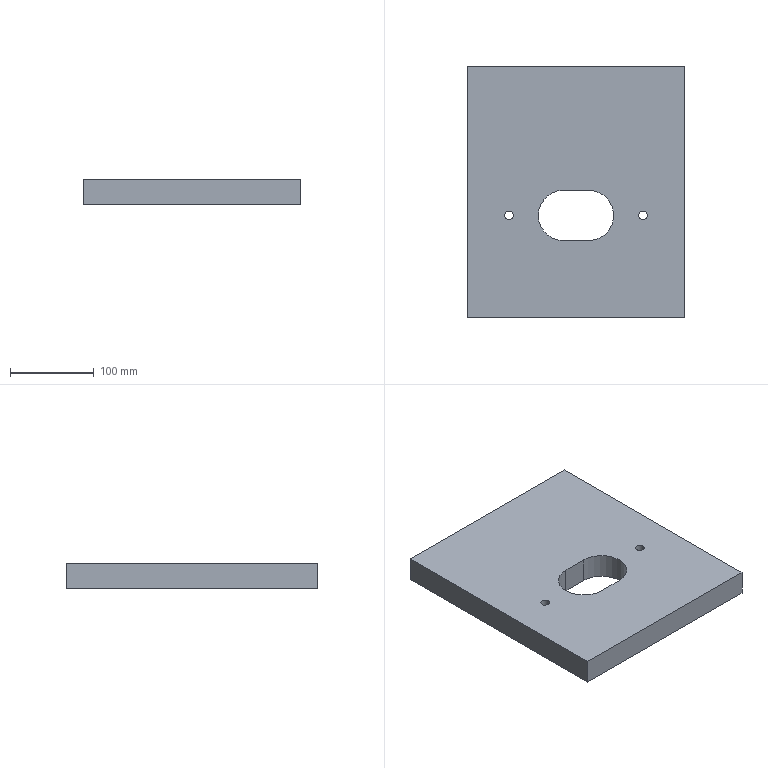Part | SolidWorks | features 3DProfileFeature 1, Extrusion 1, HoleWzd 1 | 1 solid | 15 faces | box 260 x 300 x 30 mm | volume 2196274 mm3 | plane 8 | cylinder 7 | commonest cylinder face diameters 10.2 x4 60 x3
STEP:
#1=CARTESIAN_POINT('',(44.9,122.,0.));
#2=VERTEX_POINT('',#1);
#3=CARTESIAN_POINT('',(55.1,122.,0.));
#4=VERTEX_POINT('',#3);
#5=CARTESIAN_POINT('',(50.,122.,0.));
#6=DIRECTION('',(0.,0.,1.));
#7=DIRECTION('',(1.,0.,0.));
#8=AXIS2_PLACEMENT_3D('',#5,#6,#7);
#9=CIRCLE('',#8,5.1);
#10=EDGE_CURVE('',#2,#4,#9,.T.);
#11=ORIENTED_EDGE('',*,*,#10,.F.);
#12=CARTESIAN_POINT('',(44.9,122.,30.));
#13=VERTEX_POINT('',#12);
#14=CARTESIAN_POINT('',(44.9,122.,30.));
#15=DIRECTION('',(0.,0.,1.));
#16=VECTOR('',#15,1000.);
#17=LINE('',#14,#16);
#18=EDGE_CURVE('',#2,#13,#17,.T.);
#19=ORIENTED_EDGE('',*,*,#18,.T.);
#20=CARTESIAN_POINT('',(55.1,122.,30.));
#21=VERTEX_POINT('',#20);
#22=CARTESIAN_POINT('',(50.,122.,30.));
#23=DIRECTION('',(0.,0.,1.));
#24=DIRECTION('',(1.,0.,0.));
#25=AXIS2_PLACEMENT_3D('',#22,#23,#24);
#26=CIRCLE('',#25,5.1);
#27=EDGE_CURVE('',#13,#21,#26,.T.);
#28=ORIENTED_EDGE('',*,*,#27,.T.);
#29=CARTESIAN_POINT('',(55.1,122.,30.));
#30=DIRECTION('',(0.,0.,1.));
#31=VECTOR('',#30,1000.);
#32=LINE('',#29,#31);
#33=EDGE_CURVE('',#4,#21,#32,.T.);
#34=ORIENTED_EDGE('',*,*,#33,.F.);
#35=EDGE_LOOP('',(#11,#19,#28,#34));
#36=FACE_OUTER_BOUND('',#35,.T.);
#37=CARTESIAN_POINT('',(50.,122.,30.));
#38=DIRECTION('',(0.,0.,1.));
#39=DIRECTION('',(1.,0.,0.));
#40=AXIS2_PLACEMENT_3D('',#37,#38,#39);
#41=CYLINDRICAL_SURFACE('',#40,5.1);
#42=ADVANCED_FACE('',(#36),#41,.F.);
#43=CARTESIAN_POINT('',(204.9,122.,0.));
#44=VERTEX_POINT('',#43);
#45=CARTESIAN_POINT('',(215.1,122.,0.));
#46=VERTEX_POINT('',#45);
#47=CARTESIAN_POINT('',(210.,122.,0.));
#48=DIRECTION('',(0.,0.,1.));
#49=DIRECTION('',(1.,0.,0.));
#50=AXIS2_PLACEMENT_3D('',#47,#48,#49);
#51=CIRCLE('',#50,5.1);
#52=EDGE_CURVE('',#44,#46,#51,.T.);
#53=ORIENTED_EDGE('',*,*,#52,.F.);
#54=CARTESIAN_POINT('',(204.9,122.,30.));
#55=VERTEX_POINT('',#54);
#56=CARTESIAN_POINT('',(204.9,122.,30.));
#57=DIRECTION('',(0.,0.,1.));
#58=VECTOR('',#57,1000.);
#59=LINE('',#56,#58);
#60=EDGE_CURVE('',#44,#55,#59,.T.);
#61=ORIENTED_EDGE('',*,*,#60,.T.);
#62=CARTESIAN_POINT('',(215.1,122.,30.));
#63=VERTEX_POINT('',#62);
#64=CARTESIAN_POINT('',(210.,122.,30.));
#65=DIRECTION('',(0.,0.,1.));
#66=DIRECTION('',(1.,0.,0.));
#67=AXIS2_PLACEMENT_3D('',#64,#65,#66);
#68=CIRCLE('',#67,5.1);
#69=EDGE_CURVE('',#55,#63,#68,.T.);
#70=ORIENTED_EDGE('',*,*,#69,.T.);
#71=CARTESIAN_POINT('',(215.1,122.,30.));
#72=DIRECTION('',(0.,0.,1.));
#73=VECTOR('',#72,1000.);
#74=LINE('',#71,#73);
#75=EDGE_CURVE('',#46,#63,#74,.T.);
#76=ORIENTED_EDGE('',*,*,#75,.F.);
#77=EDGE_LOOP('',(#53,#61,#70,#76));
#78=FACE_OUTER_BOUND('',#77,.T.);
#79=CARTESIAN_POINT('',(210.,122.,30.));
#80=DIRECTION('',(0.,0.,1.));
#81=DIRECTION('',(1.,0.,0.));
#82=AXIS2_PLACEMENT_3D('',#79,#80,#81);
#83=CYLINDRICAL_SURFACE('',#82,5.1);
#84=ADVANCED_FACE('',(#78),#83,.F.);
#85=CARTESIAN_POINT('',(115.,152.,30.));
#86=VERTEX_POINT('',#85);
#87=CARTESIAN_POINT('',(85.,122.,30.));
#88=VERTEX_POINT('',#87);
#89=CARTESIAN_POINT('',(115.,122.,30.));
#90=DIRECTION('',(0.,0.,1.));
#91=DIRECTION('',(1.,0.,0.));
#92=AXIS2_PLACEMENT_3D('',#89,#90,#91);
#93=CIRCLE('',#92,30.);
#94=EDGE_CURVE('',#86,#88,#93,.T.);
#95=ORIENTED_EDGE('',*,*,#94,.T.);
#96=CARTESIAN_POINT('',(85.,122.,0.));
#97=VERTEX_POINT('',#96);
#98=CARTESIAN_POINT('',(85.,122.,30.));
#99=DIRECTION('',(0.,0.,-1.));
#100=VECTOR('',#99,1000.);
#101=LINE('',#98,#100);
#102=EDGE_CURVE('',#88,#97,#101,.T.);
#103=ORIENTED_EDGE('',*,*,#102,.T.);
#104=CARTESIAN_POINT('',(115.,152.,0.));
#105=VERTEX_POINT('',#104);
#106=CARTESIAN_POINT('',(115.,122.,0.));
#107=DIRECTION('',(0.,0.,1.));
#108=DIRECTION('',(1.,0.,0.));
#109=AXIS2_PLACEMENT_3D('',#106,#107,#108);
#110=CIRCLE('',#109,30.);
#111=EDGE_CURVE('',#105,#97,#110,.T.);
#112=ORIENTED_EDGE('',*,*,#111,.F.);
#113=CARTESIAN_POINT('',(115.,152.,30.));
#114=DIRECTION('',(0.,0.,-1.));
#115=VECTOR('',#114,1000.);
#116=LINE('',#113,#115);
#117=EDGE_CURVE('',#86,#105,#116,.T.);
#118=ORIENTED_EDGE('',*,*,#117,.F.);
#119=EDGE_LOOP('',(#95,#103,#112,#118));
#120=FACE_OUTER_BOUND('',#119,.T.);
#121=CARTESIAN_POINT('',(115.,122.,30.));
#122=DIRECTION('',(0.,0.,-1.));
#123=DIRECTION('',(-1.,0.,0.));
#124=AXIS2_PLACEMENT_3D('',#121,#122,#123);
#125=CYLINDRICAL_SURFACE('',#124,30.);
#126=ADVANCED_FACE('',(#120),#125,.F.);
#127=CARTESIAN_POINT('',(50.,122.,30.));
#128=DIRECTION('',(0.,0.,1.));
#129=DIRECTION('',(1.,0.,0.));
#130=AXIS2_PLACEMENT_3D('',#127,#128,#129);
#131=CIRCLE('',#130,5.1);
#132=EDGE_CURVE('',#21,#13,#131,.T.);
#133=ORIENTED_EDGE('',*,*,#132,.F.);
#134=ORIENTED_EDGE('',*,*,#27,.F.);
#135=EDGE_LOOP('',(#133,#134));
#136=FACE_BOUND('',#135,.T.);
#137=CARTESIAN_POINT('',(210.,122.,30.));
#138=DIRECTION('',(0.,0.,1.));
#139=DIRECTION('',(1.,0.,0.));
#140=AXIS2_PLACEMENT_3D('',#137,#138,#139);
#141=CIRCLE('',#140,5.1);
#142=EDGE_CURVE('',#63,#55,#141,.T.);
#143=ORIENTED_EDGE('',*,*,#142,.F.);
#144=ORIENTED_EDGE('',*,*,#69,.F.);
#145=EDGE_LOOP('',(#143,#144));
#146=FACE_BOUND('',#145,.T.);
#147=CARTESIAN_POINT('',(0.,300.,30.));
#148=VERTEX_POINT('',#147);
#149=CARTESIAN_POINT('',(0.,0.,30.));
#150=VERTEX_POINT('',#149);
#151=CARTESIAN_POINT('',(0.,0.,30.));
#152=DIRECTION('',(0.,-1.,0.));
#153=VECTOR('',#152,1000.);
#154=LINE('',#151,#153);
#155=EDGE_CURVE('',#148,#150,#154,.T.);
#156=ORIENTED_EDGE('',*,*,#155,.T.);
#157=CARTESIAN_POINT('',(260.,0.,30.));
#158=VERTEX_POINT('',#157);
#159=CARTESIAN_POINT('',(0.,0.,30.));
#160=DIRECTION('',(1.,0.,0.));
#161=VECTOR('',#160,1000.);
#162=LINE('',#159,#161);
#163=EDGE_CURVE('',#150,#158,#162,.T.);
#164=ORIENTED_EDGE('',*,*,#163,.T.);
#165=CARTESIAN_POINT('',(260.,300.,30.));
#166=VERTEX_POINT('',#165);
#167=CARTESIAN_POINT('',(260.,0.,30.));
#168=DIRECTION('',(0.,1.,0.));
#169=VECTOR('',#168,1000.);
#170=LINE('',#167,#169);
#171=EDGE_CURVE('',#158,#166,#170,.T.);
#172=ORIENTED_EDGE('',*,*,#171,.T.);
#173=CARTESIAN_POINT('',(0.,300.,30.));
#174=DIRECTION('',(-1.,0.,0.));
#175=VECTOR('',#174,1000.);
#176=LINE('',#173,#175);
#177=EDGE_CURVE('',#166,#148,#176,.T.);
#178=ORIENTED_EDGE('',*,*,#177,.T.);
#179=EDGE_LOOP('',(#156,#164,#172,#178));
#180=FACE_OUTER_BOUND('',#179,.T.);
#181=ORIENTED_EDGE('',*,*,#94,.F.);
#182=CARTESIAN_POINT('',(145.,152.,30.));
#183=VERTEX_POINT('',#182);
#184=CARTESIAN_POINT('',(115.,152.,30.));
#185=DIRECTION('',(-1.,0.,0.));
#186=VECTOR('',#185,1000.);
#187=LINE('',#184,#186);
#188=EDGE_CURVE('',#183,#86,#187,.T.);
#189=ORIENTED_EDGE('',*,*,#188,.F.);
#190=CARTESIAN_POINT('',(145.,92.,30.));
#191=VERTEX_POINT('',#190);
#192=CARTESIAN_POINT('',(145.,122.,30.));
#193=DIRECTION('',(0.,0.,1.));
#194=DIRECTION('',(1.,0.,0.));
#195=AXIS2_PLACEMENT_3D('',#192,#193,#194);
#196=CIRCLE('',#195,30.);
#197=EDGE_CURVE('',#191,#183,#196,.T.);
#198=ORIENTED_EDGE('',*,*,#197,.F.);
#199=CARTESIAN_POINT('',(115.,92.,30.));
#200=VERTEX_POINT('',#199);
#201=CARTESIAN_POINT('',(115.,92.,30.));
#202=DIRECTION('',(1.,0.,0.));
#203=VECTOR('',#202,1000.);
#204=LINE('',#201,#203);
#205=EDGE_CURVE('',#200,#191,#204,.T.);
#206=ORIENTED_EDGE('',*,*,#205,.F.);
#207=CARTESIAN_POINT('',(115.,122.,30.));
#208=DIRECTION('',(0.,0.,1.));
#209=DIRECTION('',(1.,0.,0.));
#210=AXIS2_PLACEMENT_3D('',#207,#208,#209);
#211=CIRCLE('',#210,30.);
#212=EDGE_CURVE('',#88,#200,#211,.T.);
#213=ORIENTED_EDGE('',*,*,#212,.F.);
#214=EDGE_LOOP('',(#181,#189,#198,#206,#213));
#215=FACE_BOUND('',#214,.T.);
#216=CARTESIAN_POINT('',(0.,0.,30.));
#217=DIRECTION('',(0.,0.,-1.));
#218=DIRECTION('',(-1.,0.,0.));
#219=AXIS2_PLACEMENT_3D('',#216,#217,#218);
#220=PLANE('',#219);
#221=ADVANCED_FACE('',(#136,#146,#180,#215),#220,.F.);
#222=CARTESIAN_POINT('',(50.,122.,0.));
#223=DIRECTION('',(0.,0.,1.));
#224=DIRECTION('',(1.,0.,0.));
#225=AXIS2_PLACEMENT_3D('',#222,#223,#224);
#226=CIRCLE('',#225,5.1);
#227=EDGE_CURVE('',#4,#2,#226,.T.);
#228=ORIENTED_EDGE('',*,*,#227,.T.);
#229=ORIENTED_EDGE('',*,*,#10,.T.);
#230=EDGE_LOOP('',(#228,#229));
#231=FACE_BOUND('',#230,.T.);
#232=CARTESIAN_POINT('',(210.,122.,0.));
#233=DIRECTION('',(0.,0.,1.));
#234=DIRECTION('',(1.,0.,0.));
#235=AXIS2_PLACEMENT_3D('',#232,#233,#234);
#236=CIRCLE('',#235,5.1);
#237=EDGE_CURVE('',#46,#44,#236,.T.);
#238=ORIENTED_EDGE('',*,*,#237,.T.);
#239=ORIENTED_EDGE('',*,*,#52,.T.);
#240=EDGE_LOOP('',(#238,#239));
#241=FACE_BOUND('',#240,.T.);
#242=CARTESIAN_POINT('',(0.,300.,0.));
#243=VERTEX_POINT('',#242);
#244=CARTESIAN_POINT('',(0.,0.,0.));
#245=VERTEX_POINT('',#244);
#246=CARTESIAN_POINT('',(0.,0.,0.));
#247=DIRECTION('',(0.,-1.,0.));
#248=VECTOR('',#247,1000.);
#249=LINE('',#246,#248);
#250=EDGE_CURVE('',#243,#245,#249,.T.);
#251=ORIENTED_EDGE('',*,*,#250,.F.);
#252=CARTESIAN_POINT('',(260.,300.,0.));
#253=VERTEX_POINT('',#252);
#254=CARTESIAN_POINT('',(0.,300.,0.));
#255=DIRECTION('',(-1.,0.,0.));
#256=VECTOR('',#255,1000.);
#257=LINE('',#254,#256);
#258=EDGE_CURVE('',#253,#243,#257,.T.);
#259=ORIENTED_EDGE('',*,*,#258,.F.);
#260=CARTESIAN_POINT('',(260.,0.,0.));
#261=VERTEX_POINT('',#260);
#262=CARTESIAN_POINT('',(260.,0.,0.));
#263=DIRECTION('',(0.,1.,0.));
#264=VECTOR('',#263,1000.);
#265=LINE('',#262,#264);
#266=EDGE_CURVE('',#261,#253,#265,.T.);
#267=ORIENTED_EDGE('',*,*,#266,.F.);
#268=CARTESIAN_POINT('',(0.,0.,0.));
#269=DIRECTION('',(1.,0.,0.));
#270=VECTOR('',#269,1000.);
#271=LINE('',#268,#270);
#272=EDGE_CURVE('',#245,#261,#271,.T.);
#273=ORIENTED_EDGE('',*,*,#272,.F.);
#274=EDGE_LOOP('',(#251,#259,#267,#273));
#275=FACE_OUTER_BOUND('',#274,.T.);
#276=CARTESIAN_POINT('',(145.,152.,0.));
#277=VERTEX_POINT('',#276);
#278=CARTESIAN_POINT('',(115.,152.,0.));
#279=DIRECTION('',(-1.,0.,0.));
#280=VECTOR('',#279,1000.);
#281=LINE('',#278,#280);
#282=EDGE_CURVE('',#277,#105,#281,.T.);
#283=ORIENTED_EDGE('',*,*,#282,.T.);
#284=ORIENTED_EDGE('',*,*,#111,.T.);
#285=CARTESIAN_POINT('',(115.,92.,0.));
#286=VERTEX_POINT('',#285);
#287=CARTESIAN_POINT('',(115.,122.,0.));
#288=DIRECTION('',(0.,0.,1.));
#289=DIRECTION('',(1.,0.,0.));
#290=AXIS2_PLACEMENT_3D('',#287,#288,#289);
#291=CIRCLE('',#290,30.);
#292=EDGE_CURVE('',#97,#286,#291,.T.);
#293=ORIENTED_EDGE('',*,*,#292,.T.);
#294=CARTESIAN_POINT('',(145.,92.,0.));
#295=VERTEX_POINT('',#294);
#296=CARTESIAN_POINT('',(115.,92.,0.));
#297=DIRECTION('',(1.,0.,0.));
#298=VECTOR('',#297,1000.);
#299=LINE('',#296,#298);
#300=EDGE_CURVE('',#286,#295,#299,.T.);
#301=ORIENTED_EDGE('',*,*,#300,.T.);
#302=CARTESIAN_POINT('',(145.,122.,0.));
#303=DIRECTION('',(0.,0.,1.));
#304=DIRECTION('',(1.,0.,0.));
#305=AXIS2_PLACEMENT_3D('',#302,#303,#304);
#306=CIRCLE('',#305,30.);
#307=EDGE_CURVE('',#295,#277,#306,.T.);
#308=ORIENTED_EDGE('',*,*,#307,.T.);
#309=EDGE_LOOP('',(#283,#284,#293,#301,#308));
#310=FACE_BOUND('',#309,.T.);
#311=CARTESIAN_POINT('',(0.,0.,0.));
#312=DIRECTION('',(0.,0.,-1.));
#313=DIRECTION('',(-1.,0.,0.));
#314=AXIS2_PLACEMENT_3D('',#311,#312,#313);
#315=PLANE('',#314);
#316=ADVANCED_FACE('',(#231,#241,#275,#310),#315,.T.);
#317=ORIENTED_EDGE('',*,*,#250,.T.);
#318=CARTESIAN_POINT('',(0.,0.,30.));
#319=DIRECTION('',(0.,0.,-1.));
#320=VECTOR('',#319,1000.);
#321=LINE('',#318,#320);
#322=EDGE_CURVE('',#150,#245,#321,.T.);
#323=ORIENTED_EDGE('',*,*,#322,.F.);
#324=ORIENTED_EDGE('',*,*,#155,.F.);
#325=CARTESIAN_POINT('',(0.,300.,30.));
#326=DIRECTION('',(0.,0.,-1.));
#327=VECTOR('',#326,1000.);
#328=LINE('',#325,#327);
#329=EDGE_CURVE('',#148,#243,#328,.T.);
#330=ORIENTED_EDGE('',*,*,#329,.T.);
#331=EDGE_LOOP('',(#317,#323,#324,#330));
#332=FACE_OUTER_BOUND('',#331,.T.);
#333=CARTESIAN_POINT('',(0.,0.,30.));
#334=DIRECTION('',(1.,0.,0.));
#335=DIRECTION('',(0.,0.,-1.));
#336=AXIS2_PLACEMENT_3D('',#333,#334,#335);
#337=PLANE('',#336);
#338=ADVANCED_FACE('',(#332),#337,.F.);
#339=ORIENTED_EDGE('',*,*,#272,.T.);
#340=CARTESIAN_POINT('',(260.,0.,30.));
#341=DIRECTION('',(0.,0.,-1.));
#342=VECTOR('',#341,1000.);
#343=LINE('',#340,#342);
#344=EDGE_CURVE('',#158,#261,#343,.T.);
#345=ORIENTED_EDGE('',*,*,#344,.F.);
#346=ORIENTED_EDGE('',*,*,#163,.F.);
#347=ORIENTED_EDGE('',*,*,#322,.T.);
#348=EDGE_LOOP('',(#339,#345,#346,#347));
#349=FACE_OUTER_BOUND('',#348,.T.);
#350=CARTESIAN_POINT('',(0.,0.,30.));
#351=DIRECTION('',(0.,1.,0.));
#352=DIRECTION('',(0.,0.,1.));
#353=AXIS2_PLACEMENT_3D('',#350,#351,#352);
#354=PLANE('',#353);
#355=ADVANCED_FACE('',(#349),#354,.F.);
#356=ORIENTED_EDGE('',*,*,#266,.T.);
#357=CARTESIAN_POINT('',(260.,300.,30.));
#358=DIRECTION('',(0.,0.,-1.));
#359=VECTOR('',#358,1000.);
#360=LINE('',#357,#359);
#361=EDGE_CURVE('',#166,#253,#360,.T.);
#362=ORIENTED_EDGE('',*,*,#361,.F.);
#363=ORIENTED_EDGE('',*,*,#171,.F.);
#364=ORIENTED_EDGE('',*,*,#344,.T.);
#365=EDGE_LOOP('',(#356,#362,#363,#364));
#366=FACE_OUTER_BOUND('',#365,.T.);
#367=CARTESIAN_POINT('',(260.,0.,30.));
#368=DIRECTION('',(-1.,0.,0.));
#369=DIRECTION('',(0.,0.,1.));
#370=AXIS2_PLACEMENT_3D('',#367,#368,#369);
#371=PLANE('',#370);
#372=ADVANCED_FACE('',(#366),#371,.F.);
#373=ORIENTED_EDGE('',*,*,#258,.T.);
#374=ORIENTED_EDGE('',*,*,#329,.F.);
#375=ORIENTED_EDGE('',*,*,#177,.F.);
#376=ORIENTED_EDGE('',*,*,#361,.T.);
#377=EDGE_LOOP('',(#373,#374,#375,#376));
#378=FACE_OUTER_BOUND('',#377,.T.);
#379=CARTESIAN_POINT('',(0.,300.,30.));
#380=DIRECTION('',(0.,-1.,0.));
#381=DIRECTION('',(0.,0.,-1.));
#382=AXIS2_PLACEMENT_3D('',#379,#380,#381);
#383=PLANE('',#382);
#384=ADVANCED_FACE('',(#378),#383,.F.);
#385=ORIENTED_EDGE('',*,*,#102,.F.);
#386=ORIENTED_EDGE('',*,*,#212,.T.);
#387=CARTESIAN_POINT('',(115.,92.,30.));
#388=DIRECTION('',(0.,0.,-1.));
#389=VECTOR('',#388,1000.);
#390=LINE('',#387,#389);
#391=EDGE_CURVE('',#200,#286,#390,.T.);
#392=ORIENTED_EDGE('',*,*,#391,.T.);
#393=ORIENTED_EDGE('',*,*,#292,.F.);
#394=EDGE_LOOP('',(#385,#386,#392,#393));
#395=FACE_OUTER_BOUND('',#394,.T.);
#396=CARTESIAN_POINT('',(115.,122.,30.));
#397=DIRECTION('',(0.,0.,-1.));
#398=DIRECTION('',(-1.,0.,0.));
#399=AXIS2_PLACEMENT_3D('',#396,#397,#398);
#400=CYLINDRICAL_SURFACE('',#399,30.);
#401=ADVANCED_FACE('',(#395),#400,.F.);
#402=ORIENTED_EDGE('',*,*,#300,.F.);
#403=ORIENTED_EDGE('',*,*,#391,.F.);
#404=ORIENTED_EDGE('',*,*,#205,.T.);
#405=CARTESIAN_POINT('',(145.,92.,30.));
#406=DIRECTION('',(0.,0.,-1.));
#407=VECTOR('',#406,1000.);
#408=LINE('',#405,#407);
#409=EDGE_CURVE('',#191,#295,#408,.T.);
#410=ORIENTED_EDGE('',*,*,#409,.T.);
#411=EDGE_LOOP('',(#402,#403,#404,#410));
#412=FACE_OUTER_BOUND('',#411,.T.);
#413=CARTESIAN_POINT('',(115.,92.,30.));
#414=DIRECTION('',(0.,1.,0.));
#415=DIRECTION('',(0.,0.,1.));
#416=AXIS2_PLACEMENT_3D('',#413,#414,#415);
#417=PLANE('',#416);
#418=ADVANCED_FACE('',(#412),#417,.T.);
#419=ORIENTED_EDGE('',*,*,#307,.F.);
#420=ORIENTED_EDGE('',*,*,#409,.F.);
#421=ORIENTED_EDGE('',*,*,#197,.T.);
#422=CARTESIAN_POINT('',(145.,152.,30.));
#423=DIRECTION('',(0.,0.,-1.));
#424=VECTOR('',#423,1000.);
#425=LINE('',#422,#424);
#426=EDGE_CURVE('',#183,#277,#425,.T.);
#427=ORIENTED_EDGE('',*,*,#426,.T.);
#428=EDGE_LOOP('',(#419,#420,#421,#427));
#429=FACE_OUTER_BOUND('',#428,.T.);
#430=CARTESIAN_POINT('',(145.,122.,30.));
#431=DIRECTION('',(0.,0.,-1.));
#432=DIRECTION('',(-1.,0.,0.));
#433=AXIS2_PLACEMENT_3D('',#430,#431,#432);
#434=CYLINDRICAL_SURFACE('',#433,30.);
#435=ADVANCED_FACE('',(#429),#434,.F.);
#436=ORIENTED_EDGE('',*,*,#282,.F.);
#437=ORIENTED_EDGE('',*,*,#426,.F.);
#438=ORIENTED_EDGE('',*,*,#188,.T.);
#439=ORIENTED_EDGE('',*,*,#117,.T.);
#440=EDGE_LOOP('',(#436,#437,#438,#439));
#441=FACE_OUTER_BOUND('',#440,.T.);
#442=CARTESIAN_POINT('',(115.,152.,30.));
#443=DIRECTION('',(0.,-1.,0.));
#444=DIRECTION('',(0.,0.,-1.));
#445=AXIS2_PLACEMENT_3D('',#442,#443,#444);
#446=PLANE('',#445);
#447=ADVANCED_FACE('',(#441),#446,.T.);
#448=ORIENTED_EDGE('',*,*,#60,.F.);
#449=ORIENTED_EDGE('',*,*,#237,.F.);
#450=ORIENTED_EDGE('',*,*,#75,.T.);
#451=ORIENTED_EDGE('',*,*,#142,.T.);
#452=EDGE_LOOP('',(#448,#449,#450,#451));
#453=FACE_OUTER_BOUND('',#452,.T.);
#454=CARTESIAN_POINT('',(210.,122.,30.));
#455=DIRECTION('',(0.,0.,1.));
#456=DIRECTION('',(1.,0.,0.));
#457=AXIS2_PLACEMENT_3D('',#454,#455,#456);
#458=CYLINDRICAL_SURFACE('',#457,5.1);
#459=ADVANCED_FACE('',(#453),#458,.F.);
#460=ORIENTED_EDGE('',*,*,#18,.F.);
#461=ORIENTED_EDGE('',*,*,#227,.F.);
#462=ORIENTED_EDGE('',*,*,#33,.T.);
#463=ORIENTED_EDGE('',*,*,#132,.T.);
#464=EDGE_LOOP('',(#460,#461,#462,#463));
#465=FACE_OUTER_BOUND('',#464,.T.);
#466=CARTESIAN_POINT('',(50.,122.,30.));
#467=DIRECTION('',(0.,0.,1.));
#468=DIRECTION('',(1.,0.,0.));
#469=AXIS2_PLACEMENT_3D('',#466,#467,#468);
#470=CYLINDRICAL_SURFACE('',#469,5.1);
#471=ADVANCED_FACE('',(#465),#470,.F.);
#472=CLOSED_SHELL('',(#42,#84,#126,#221,#316,#338,#355,#372,#384,#401,#418,#435,#447,#459,#471));
#473=MANIFOLD_SOLID_BREP('',#472);
#474=CARTESIAN_POINT('',(0.,0.,0.));
#475=DIRECTION('',(0.,0.,1.));
#476=DIRECTION('',(1.,0.,0.));
#477=AXIS2_PLACEMENT_3D('',#474,#475,#476);
#478=(LENGTH_UNIT()NAMED_UNIT(*)SI_UNIT(.MILLI.,.METRE.));
#479=UNCERTAINTY_MEASURE_WITH_UNIT(LENGTH_MEASURE(0.00001),#478,'','');
#480=(NAMED_UNIT(*)PLANE_ANGLE_UNIT()SI_UNIT($,.RADIAN.));
#481=(NAMED_UNIT(*)SI_UNIT($,.STERADIAN.)SOLID_ANGLE_UNIT());
#482=(GEOMETRIC_REPRESENTATION_CONTEXT(3)GLOBAL_UNCERTAINTY_ASSIGNED_CONTEXT((#479))GLOBAL_UNIT_ASSIGNED_CONTEXT((#478,#480,#481))REPRESENTATION_CONTEXT('',''));
#483=ADVANCED_BREP_SHAPE_REPRESENTATION('',(#473,#477),#482);